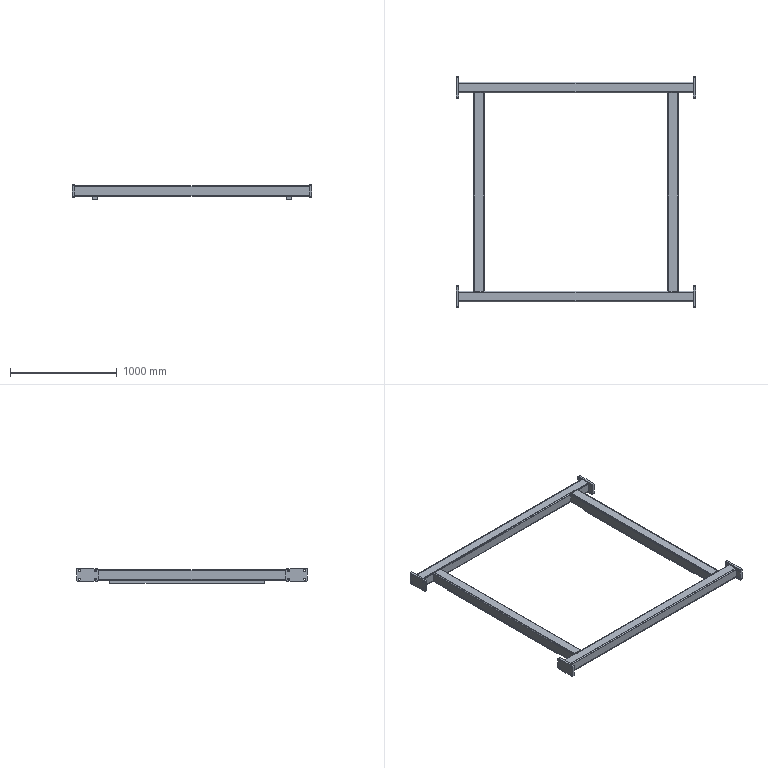Part | STEP file | 10 solids | 156 faces | box 2240 x 2160 x 139 mm | volume 20941933 mm3 | cylinder 80 | plane 76 | commonest cylinder face diameters 18 x32 20 x32 10 x16